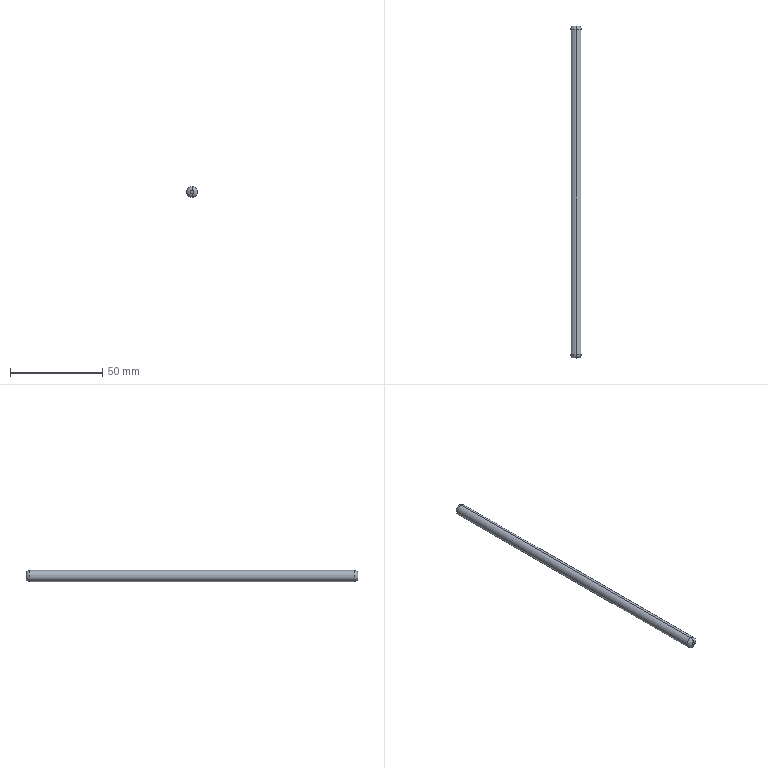Part | SolidWorks | features Extrusion 1, Fillet 1 | 1 solid | 8 faces | box 6 x 180 x 6 mm | volume 5062 mm3 | torus 4 | cylinder 2 | plane 2 | commonest cylinder face diameters 6 x2
STEP:
#1=CARTESIAN_POINT('',(0.,178.,-3.));
#2=VERTEX_POINT('',#1);
#3=CARTESIAN_POINT('',(0.,178.,3.));
#4=VERTEX_POINT('',#3);
#5=CARTESIAN_POINT('',(0.,178.,0.));
#6=DIRECTION('',(0.,-1.,0.));
#7=DIRECTION('',(0.,0.,1.));
#8=AXIS2_PLACEMENT_3D('',#5,#6,#7);
#9=CIRCLE('',#8,3.);
#10=EDGE_CURVE('',#2,#4,#9,.T.);
#11=ORIENTED_EDGE('',*,*,#10,.F.);
#12=CARTESIAN_POINT('',(0.,180.,-1.));
#13=VERTEX_POINT('',#12);
#14=CARTESIAN_POINT('',(0.,178.,-1.));
#15=DIRECTION('',(1.,0.,0.));
#16=DIRECTION('',(0.,0.,-1.));
#17=AXIS2_PLACEMENT_3D('',#14,#15,#16);
#18=CIRCLE('',#17,2.);
#19=EDGE_CURVE('',#2,#13,#18,.T.);
#20=ORIENTED_EDGE('',*,*,#19,.T.);
#21=CARTESIAN_POINT('',(0.,180.,1.));
#22=VERTEX_POINT('',#21);
#23=CARTESIAN_POINT('',(0.,180.,0.));
#24=DIRECTION('',(0.,1.,0.));
#25=DIRECTION('',(0.,0.,1.));
#26=AXIS2_PLACEMENT_3D('',#23,#24,#25);
#27=CIRCLE('',#26,1.);
#28=EDGE_CURVE('',#22,#13,#27,.T.);
#29=ORIENTED_EDGE('',*,*,#28,.F.);
#30=CARTESIAN_POINT('',(0.,178.,1.));
#31=DIRECTION('',(-1.,0.,0.));
#32=DIRECTION('',(0.,0.,1.));
#33=AXIS2_PLACEMENT_3D('',#30,#31,#32);
#34=CIRCLE('',#33,2.);
#35=EDGE_CURVE('',#4,#22,#34,.T.);
#36=ORIENTED_EDGE('',*,*,#35,.F.);
#37=EDGE_LOOP('',(#11,#20,#29,#36));
#38=FACE_OUTER_BOUND('',#37,.T.);
#39=CARTESIAN_POINT('',(0.,178.,0.));
#40=DIRECTION('',(0.,1.,0.));
#41=DIRECTION('',(0.,0.,1.));
#42=AXIS2_PLACEMENT_3D('',#39,#40,#41);
#43=TOROIDAL_SURFACE('',#42,1.,2.);
#44=ADVANCED_FACE('',(#38),#43,.T.);
#45=CARTESIAN_POINT('',(0.,0.,-1.));
#46=VERTEX_POINT('',#45);
#47=CARTESIAN_POINT('',(0.,0.,1.));
#48=VERTEX_POINT('',#47);
#49=CARTESIAN_POINT('',(0.,0.,0.));
#50=DIRECTION('',(0.,-1.,0.));
#51=DIRECTION('',(0.,0.,1.));
#52=AXIS2_PLACEMENT_3D('',#49,#50,#51);
#53=CIRCLE('',#52,1.);
#54=EDGE_CURVE('',#46,#48,#53,.T.);
#55=ORIENTED_EDGE('',*,*,#54,.F.);
#56=CARTESIAN_POINT('',(0.,2.,-3.));
#57=VERTEX_POINT('',#56);
#58=CARTESIAN_POINT('',(0.,2.,-1.));
#59=DIRECTION('',(1.,0.,0.));
#60=DIRECTION('',(0.,0.,-1.));
#61=AXIS2_PLACEMENT_3D('',#58,#59,#60);
#62=CIRCLE('',#61,2.);
#63=EDGE_CURVE('',#46,#57,#62,.T.);
#64=ORIENTED_EDGE('',*,*,#63,.T.);
#65=CARTESIAN_POINT('',(0.,2.,3.));
#66=VERTEX_POINT('',#65);
#67=CARTESIAN_POINT('',(0.,2.,0.));
#68=DIRECTION('',(0.,1.,0.));
#69=DIRECTION('',(0.,0.,1.));
#70=AXIS2_PLACEMENT_3D('',#67,#68,#69);
#71=CIRCLE('',#70,3.);
#72=EDGE_CURVE('',#66,#57,#71,.T.);
#73=ORIENTED_EDGE('',*,*,#72,.F.);
#74=CARTESIAN_POINT('',(0.,2.,1.));
#75=DIRECTION('',(-1.,0.,0.));
#76=DIRECTION('',(0.,0.,1.));
#77=AXIS2_PLACEMENT_3D('',#74,#75,#76);
#78=CIRCLE('',#77,2.);
#79=EDGE_CURVE('',#48,#66,#78,.T.);
#80=ORIENTED_EDGE('',*,*,#79,.F.);
#81=EDGE_LOOP('',(#55,#64,#73,#80));
#82=FACE_OUTER_BOUND('',#81,.T.);
#83=CARTESIAN_POINT('',(0.,2.,0.));
#84=DIRECTION('',(0.,1.,0.));
#85=DIRECTION('',(0.,0.,1.));
#86=AXIS2_PLACEMENT_3D('',#83,#84,#85);
#87=TOROIDAL_SURFACE('',#86,1.,2.);
#88=ADVANCED_FACE('',(#82),#87,.T.);
#89=ORIENTED_EDGE('',*,*,#10,.T.);
#90=CARTESIAN_POINT('',(0.,180.,3.));
#91=DIRECTION('',(0.,-1.,0.));
#92=VECTOR('',#91,1000.);
#93=LINE('',#90,#92);
#94=EDGE_CURVE('',#4,#66,#93,.T.);
#95=ORIENTED_EDGE('',*,*,#94,.T.);
#96=ORIENTED_EDGE('',*,*,#72,.T.);
#97=CARTESIAN_POINT('',(0.,180.,-3.));
#98=DIRECTION('',(0.,-1.,0.));
#99=VECTOR('',#98,1000.);
#100=LINE('',#97,#99);
#101=EDGE_CURVE('',#2,#57,#100,.T.);
#102=ORIENTED_EDGE('',*,*,#101,.F.);
#103=EDGE_LOOP('',(#89,#95,#96,#102));
#104=FACE_OUTER_BOUND('',#103,.T.);
#105=CARTESIAN_POINT('',(0.,180.,0.));
#106=DIRECTION('',(0.,-1.,0.));
#107=DIRECTION('',(0.,0.,-1.));
#108=AXIS2_PLACEMENT_3D('',#105,#106,#107);
#109=CYLINDRICAL_SURFACE('',#108,3.);
#110=ADVANCED_FACE('',(#104),#109,.T.);
#111=ORIENTED_EDGE('',*,*,#94,.F.);
#112=CARTESIAN_POINT('',(0.,178.,0.));
#113=DIRECTION('',(0.,-1.,0.));
#114=DIRECTION('',(0.,0.,1.));
#115=AXIS2_PLACEMENT_3D('',#112,#113,#114);
#116=CIRCLE('',#115,3.);
#117=EDGE_CURVE('',#4,#2,#116,.T.);
#118=ORIENTED_EDGE('',*,*,#117,.T.);
#119=ORIENTED_EDGE('',*,*,#101,.T.);
#120=CARTESIAN_POINT('',(0.,2.,0.));
#121=DIRECTION('',(0.,1.,0.));
#122=DIRECTION('',(0.,0.,1.));
#123=AXIS2_PLACEMENT_3D('',#120,#121,#122);
#124=CIRCLE('',#123,3.);
#125=EDGE_CURVE('',#57,#66,#124,.T.);
#126=ORIENTED_EDGE('',*,*,#125,.T.);
#127=EDGE_LOOP('',(#111,#118,#119,#126));
#128=FACE_OUTER_BOUND('',#127,.T.);
#129=CARTESIAN_POINT('',(0.,180.,0.));
#130=DIRECTION('',(0.,-1.,0.));
#131=DIRECTION('',(0.,0.,-1.));
#132=AXIS2_PLACEMENT_3D('',#129,#130,#131);
#133=CYLINDRICAL_SURFACE('',#132,3.);
#134=ADVANCED_FACE('',(#128),#133,.T.);
#135=ORIENTED_EDGE('',*,*,#28,.T.);
#136=CARTESIAN_POINT('',(0.,180.,0.));
#137=DIRECTION('',(0.,1.,0.));
#138=DIRECTION('',(0.,0.,1.));
#139=AXIS2_PLACEMENT_3D('',#136,#137,#138);
#140=CIRCLE('',#139,1.);
#141=EDGE_CURVE('',#13,#22,#140,.T.);
#142=ORIENTED_EDGE('',*,*,#141,.T.);
#143=EDGE_LOOP('',(#135,#142));
#144=FACE_OUTER_BOUND('',#143,.T.);
#145=CARTESIAN_POINT('',(0.,180.,0.));
#146=DIRECTION('',(0.,1.,0.));
#147=DIRECTION('',(0.,0.,1.));
#148=AXIS2_PLACEMENT_3D('',#145,#146,#147);
#149=PLANE('',#148);
#150=ADVANCED_FACE('',(#144),#149,.T.);
#151=CARTESIAN_POINT('',(0.,0.,0.));
#152=DIRECTION('',(0.,-1.,0.));
#153=DIRECTION('',(0.,0.,1.));
#154=AXIS2_PLACEMENT_3D('',#151,#152,#153);
#155=CIRCLE('',#154,1.);
#156=EDGE_CURVE('',#48,#46,#155,.T.);
#157=ORIENTED_EDGE('',*,*,#156,.T.);
#158=ORIENTED_EDGE('',*,*,#54,.T.);
#159=EDGE_LOOP('',(#157,#158));
#160=FACE_OUTER_BOUND('',#159,.T.);
#161=CARTESIAN_POINT('',(0.,0.,0.));
#162=DIRECTION('',(0.,1.,0.));
#163=DIRECTION('',(0.,0.,1.));
#164=AXIS2_PLACEMENT_3D('',#161,#162,#163);
#165=PLANE('',#164);
#166=ADVANCED_FACE('',(#160),#165,.F.);
#167=ORIENTED_EDGE('',*,*,#63,.F.);
#168=ORIENTED_EDGE('',*,*,#156,.F.);
#169=ORIENTED_EDGE('',*,*,#79,.T.);
#170=ORIENTED_EDGE('',*,*,#125,.F.);
#171=EDGE_LOOP('',(#167,#168,#169,#170));
#172=FACE_OUTER_BOUND('',#171,.T.);
#173=CARTESIAN_POINT('',(0.,2.,0.));
#174=DIRECTION('',(0.,1.,0.));
#175=DIRECTION('',(0.,0.,1.));
#176=AXIS2_PLACEMENT_3D('',#173,#174,#175);
#177=TOROIDAL_SURFACE('',#176,1.,2.);
#178=ADVANCED_FACE('',(#172),#177,.T.);
#179=ORIENTED_EDGE('',*,*,#19,.F.);
#180=ORIENTED_EDGE('',*,*,#117,.F.);
#181=ORIENTED_EDGE('',*,*,#35,.T.);
#182=ORIENTED_EDGE('',*,*,#141,.F.);
#183=EDGE_LOOP('',(#179,#180,#181,#182));
#184=FACE_OUTER_BOUND('',#183,.T.);
#185=CARTESIAN_POINT('',(0.,178.,0.));
#186=DIRECTION('',(0.,1.,0.));
#187=DIRECTION('',(0.,0.,1.));
#188=AXIS2_PLACEMENT_3D('',#185,#186,#187);
#189=TOROIDAL_SURFACE('',#188,1.,2.);
#190=ADVANCED_FACE('',(#184),#189,.T.);
#191=CLOSED_SHELL('',(#44,#88,#110,#134,#150,#166,#178,#190));
#192=MANIFOLD_SOLID_BREP('',#191);
#193=CARTESIAN_POINT('',(0.,0.,0.));
#194=DIRECTION('',(0.,0.,1.));
#195=DIRECTION('',(1.,0.,0.));
#196=AXIS2_PLACEMENT_3D('',#193,#194,#195);
#197=(LENGTH_UNIT()NAMED_UNIT(*)SI_UNIT(.MILLI.,.METRE.));
#198=UNCERTAINTY_MEASURE_WITH_UNIT(LENGTH_MEASURE(0.00001),#197,'','');
#199=(NAMED_UNIT(*)PLANE_ANGLE_UNIT()SI_UNIT($,.RADIAN.));
#200=(NAMED_UNIT(*)SI_UNIT($,.STERADIAN.)SOLID_ANGLE_UNIT());
#201=(GEOMETRIC_REPRESENTATION_CONTEXT(3)GLOBAL_UNCERTAINTY_ASSIGNED_CONTEXT((#198))GLOBAL_UNIT_ASSIGNED_CONTEXT((#197,#199,#200))REPRESENTATION_CONTEXT('',''));
#202=ADVANCED_BREP_SHAPE_REPRESENTATION('',(#192,#196),#201);